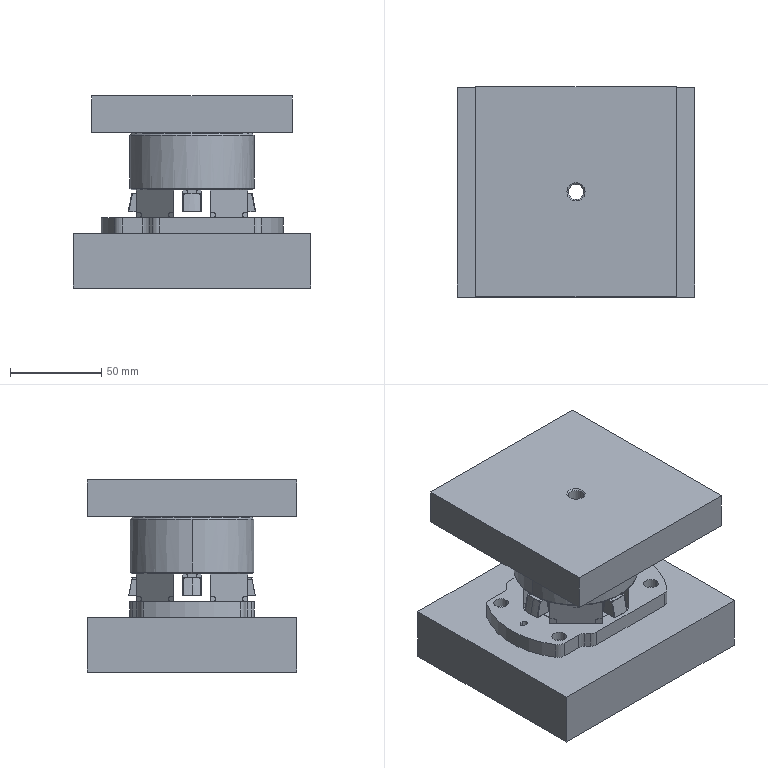NC program | NX | posted with a generic post | part box 130 x 115 x 105.2 mm
Lines 1 to 1664 of 1812, first 1463 of 1650 lines:
N10 G17 G21 G94 G90
(ADAPTIVE_MILLING_1 , TOOL : ER25-D10-50)
N12 T04 M6
N14 G54
N16 G17 G0 G90 X65.581 Y1.184 B0. C0. S6500 M3
N18 G43 Z50. H4
N20 Z-6.85
N22 G94 G1 X65.432 Y1.173 Z-7.787 F2500.
N24 X65.282 Y1.162 Z-8.158
N26 X65.133 Y1.151 Z-8.43
N28 X64.983 Y1.139 Z-8.65
N30 X64.834 Y1.128 Z-8.834
N32 X64.684 Y1.117 Z-8.992
N34 X64.534 Y1.106 Z-9.13
N36 X64.385 Y1.095 Z-9.25
N38 X64.235 Y1.084 Z-9.355
N40 X64.086 Y1.073 Z-9.448
N42 X63.936 Y1.062 Z-9.529
N44 X63.786 Y1.05 Z-9.6
N46 X63.637 Y1.039 Z-9.66
N48 X63.487 Y1.028 Z-9.712
N50 X63.338 Y1.017 Z-9.755
N52 X63.188 Y1.006 Z-9.789
N54 X63.038 Y0.995 Z-9.816
N56 X62.889 Y0.984 Z-9.835
N58 X62.739 Y0.973 Z-9.846
N60 X62.59 Y0.962 Z-9.85
N62 X60.898 Y0.836
N64 G3 X60.073 Y0.287 R1.011
N66 X59.334 Y-2.595 R8.58
N68 X59.03 Y-9.309 R68.894
N70 G1 X58.999 Y-20.218
N72 X58.998 Y-54.643
N74 G2 X57.298 Y-58.286 R5.275
N76 X53.088 Y-60.557 R9.591
N78 X47.379 Y-61.345 R26.709
N80 X37.556 Y-61.496 R223.301
N82 G1 X31.781 Y-61.5
N84 X-52.193 Y-61.498
N86 G2 X-55.736 Y-59.84 R5.295
N88 X-58.042 Y-55.63 R9.519
N90 X-58.845 Y-49.847 R26.601
N92 X-58.996 Y-39.424 R237.991
N94 G1 X-58.998 Y-34.474
N96 X-58.996 Y54.766
N98 G2 X-57.18 Y58.434 R5.368
N100 X-52.956 Y60.612 R9.75
N102 X-47.165 Y61.358 R28.291
N104 X-34.942 Y61.498 R307.021
N106 G1 X52.124 Y61.499
N108 G2 X55.836 Y59.781 R5.281
N110 X58.074 Y55.593 R9.546
N112 X58.843 Y49.956 R26.863
N114 X58.995 Y40.058 R225.033
N116 G1 X58.998 Y34.133
N118 Y3.858
N120 G2 X58.558 Y-0.729 R47.799
N122 G3 X58.039 Y-10.664 R96.401
N124 X57.999 Y-21.268 R738.972
N126 G1 X57.997 Y-51.718
N128 G2 X55.1 Y-57.334 R7.34
N130 X50.069 Y-59.612 R12.527
N132 X43.371 Y-60.37 R36.438
N134 X31.298 Y-60.498 R355.1
N136 G1 X-49.043 Y-60.499
N138 G2 X-54.865 Y-57.555 R7.352
N140 X-57.102 Y-52.6 R12.564
N142 X-57.867 Y-45.904 R36.265
N144 X-57.997 Y-33.38 R364.74
N146 G1 X-57.999 Y51.616
N148 G2 X-55.024 Y57.413 R7.314
N150 X-49.98 Y59.639 R12.698
N152 X-43.354 Y60.371 R37.226
N154 X-30.98 Y60.497 R370.258
N156 G1 X49.115 Y60.499
N158 G2 X54.867 Y57.581 R7.301
N160 X57.105 Y52.624 R12.526
N162 X57.861 Y46.077 R35.796
N164 X57.997 Y33.404 R353.751
N166 G1 X57.998 Y6.483
N168 G2 X57.547 Y-0.617 R77.039
N170 G3 X57.02 Y-14.091 R160.217
N172 G1 X57. Y-24.118
N174 X56.999 Y-48.993
N176 G2 X53.038 Y-56.516 R8.69
N178 X47.485 Y-58.685 R15.07
N180 X40.477 Y-59.377 R44.29
N182 X26.003 Y-59.498 R479.139
N184 G1 X-46.493
N186 G2 X-54.053 Y-55.478 R8.701
N188 X-56.201 Y-49.898 R15.208
N190 X-56.891 Y-42.514 R46.719
N192 X-56.997 Y-28.415 R538.22
N194 G1 Y49.066
N196 G2 X-53.012 Y56.544 R8.655
N198 X-47.599 Y58.666 R14.978
N200 X-40.443 Y59.378 R44.055
N202 X-24.694 Y59.498 R542.707
N204 G1 X46.531
N206 G2 X54.07 Y55.474 R8.673
N208 X56.194 Y49.957 R15.187
N210 X56.88 Y42.873 R45.112
N212 X56.997 Y28.399 R498.713
N214 G1 X56.995 Y8.058
N216 G2 X56.539 Y-0.562 R114.182
N218 G3 X56.012 Y-16.781 R219.905
N220 G1 X56. Y-25.018
N222 X55.999 Y-46.618
N224 G2 X55.202 Y-51.165 R11.232
N226 X50.575 Y-55.993 R10.068
N228 X44.66 Y-57.836 R18.683
N230 X36.887 Y-58.415 R60.361
N232 X22.037 Y-58.498 R765.904
N234 G1 X-44.168 Y-58.497
N236 G2 X-48.779 Y-57.649 R11.007
N238 X-53.504 Y-53.051 R10.114
N240 X-55.339 Y-47.125 R18.765
N242 X-55.921 Y-39.051 R62.317
N244 X-55.997 Y-25.852 R759.417
N246 G1 Y46.666
N248 G2 X-55.187 Y51.209 R11.083
N250 X-50.584 Y55.995 R10.052
N252 X-44.66 Y57.837 R18.699
N254 X-36.737 Y58.418 R61.322
N256 X-21.888 Y58.498 R807.199
N258 G1 X44.165 Y58.497
N260 G2 X48.709 Y57.687 R11.085
N262 X53.496 Y53.082 R10.049
N264 X55.337 Y47.158 R18.706
N266 X55.921 Y39.085 R62.102
N268 X55.997 Y25.886 R759.211
N270 G1 X55.996 Y10.011
N272 G2 X55.519 Y-0.75 R149.74
N274 G3 X55.009 Y-18.653 R271.158
N276 G1 X55. Y-26.893
N278 X54.999 Y-44.418
N280 G2 X54.496 Y-48.722 R14.697
N282 X49.785 Y-54.561 R10.27
N284 X43.719 Y-56.688 R18.043
N286 X35.807 Y-57.386 R54.254
N288 X19.683 Y-57.498 R625.027
N290 G1 X-42.017 Y-57.496
N292 G2 X-46.46 Y-56.919 R14.012
N294 X-52.181 Y-52.078 R10.365
N296 X-54.202 Y-46.131 R18.445
N298 X-54.889 Y-38.142 R55.53
N300 X-54.997 Y-22.093 R653.276
N302 G1 X-54.996 Y44.566
N304 G2 X-54.408 Y49.007 R13.879
N306 X-49.595 Y54.678 R10.344
N308 X-43.499 Y56.728 R18.571
N310 X-35.733 Y57.388 R56.178
N312 X-19.984 Y57.497 R616.787
N314 G1 X41.99
N316 G2 X46.363 Y56.955 R14.314
N318 X52.104 Y52.222 R10.284
N320 X54.202 Y46.144 R18.234
N322 X54.892 Y38.081 R55.809
N324 X54.996 Y23.682 R592.8
N326 G1 X54.995 Y11.583
N328 G2 X54.494 Y-1.098 R190.151
N330 G3 X54.007 Y-20.675 R325.437
N332 G1 X54.001 Y-27.268
N334 X54. Y-42.318
N336 G2 X53.595 Y-46.788 R18.659
N338 X48.585 Y-53.411 R10.673
N340 X42.533 Y-55.599 R18.347
N342 X34.477 Y-56.367 R52.641
N344 X17.978 Y-56.497 R567.816
N346 G1 X-40.043 Y-56.496
N348 G2 X-44.506 Y-56.036 R17.278
N350 X-50.925 Y-51.061 R10.706
N352 X-53.114 Y-44.946 R18.475
N354 X-53.863 Y-37.039 R52.944
N356 X-53.995 Y-22.566 R481.086
N358 G1 X-53.997 Y41.984
N360 G2 X-53.67 Y46.463 R21.304
N362 X-48.641 Y53.382 R10.64
N364 X-42.534 Y55.599 R18.286
N366 X-34.403 Y56.369 R53.01
N368 X-17.83 Y56.497 R581.839
N370 G1 X40.04 Y56.496
N372 G2 X44.504 Y56.041 R17.334
N374 X50.971 Y50.992 R10.714
N376 X53.132 Y44.859 R18.66
N378 X53.869 Y36.875 R54.132
N380 X53.996 Y20.002 R595.418
N382 X53.894 Y6.859 R402.358
N384 X53.332 Y-4.268 R926.663
N386 G3 X53.003 Y-23.896 R438.267
N388 G1 X53.001 Y-28.843
N390 X53. Y-40.368
N392 G2 X52.672 Y-44.923 R23.27
N394 X47.328 Y-52.337 R11.086
N396 X41.071 Y-54.58 R19.057
N398 X32.791 Y-55.363 R54.844
N400 X18.692 Y-55.496 R477.775
N402 G1 X-37.458 Y-55.497
N404 G2 X-42.168 Y-55.219 R26.666
N406 X-49.894 Y-49.73 R11.111
N408 X-52.086 Y-43.539 R19.184
N410 X-52.858 Y-35.409 R54.524
N412 X-52.995 Y-20.935 R475.03
N414 G1 X-52.996 Y40.141
N416 G2 X-52.701 Y44.774 R25.127
N418 X-47.289 Y52.363 R11.067
N420 X-41.019 Y54.591 R19.177
N422 X-32.663 Y55.367 R55.62
N424 X-15.789 Y55.496 R596.273
N426 G1 X37.961
N428 G2 X42.661 Y55.123 R21.898
N430 X49.849 Y49.812 R11.083
N432 X52.097 Y43.483 R19.174
N434 X52.86 Y35.351 R55.164
N436 X52.995 Y20.952 R480.194
N438 X52.896 Y7.553 R432.06
N440 X52.349 Y-4.038 R856.063
N442 G3 X52.003 Y-25.32 R483.268
N444 G1 X52.001 Y-37.668
N446 G2 X51.79 Y-42.759 R37.517
N448 X46.039 Y-51.312 R11.491
N450 X39.633 Y-53.572 R19.769
N452 X31.278 Y-54.358 R56.565
N454 X16.879 Y-54.495 R478.938
N456 G1 X-35.693 Y-54.496
N458 G2 X-40.63 Y-54.229 R30.471
N460 X-48.843 Y-48.484 R11.482
N462 X-51.083 Y-42.063 R19.895
N464 X-51.856 Y-33.781 R56.857
N466 X-51.995 Y-18.858 R495.156
N468 G1 X-51.996 Y37.967
N470 G2 X-51.755 Y42.981 R33.159
N472 X-46.047 Y51.309 R11.454
N474 X-39.623 Y53.573 R19.798
N476 X-31.417 Y54.352 R55.913
N478 X-16.569 Y54.495 R477.594
N480 G1 X35.69 Y54.496
N482 G2 X40.627 Y54.231 R30.554
N484 X48.809 Y48.546 R11.454
N486 X51.073 Y42.12 R19.774
N488 X51.859 Y33.69 R56.924
N490 X51.995 Y17.191 R557.858
N492 X51.491 Y-1.059 R289.671
N494 G3 X51.006 Y-23.973 R448.609
N496 G1 X51.002 Y-30.568
N498 G2 X50.955 Y-39.392 R282.827
N500 X49.869 Y-44.727 R14.734
N502 X44.416 Y-50.497 R12.086
N504 X37.952 Y-52.617 R21.22
N506 X29.367 Y-53.368 R61.75
N508 X11.668 Y-53.496 R655.381
N510 G1 X-34.432 Y-53.495
N512 G2 X-39.441 Y-53.188 R29.462
N514 X-47.818 Y-47.23 R11.811
N516 X-50.05 Y-40.812 R20.383
N518 X-50.851 Y-32.308 R57.628
N520 X-50.995 Y-15.434 R560.068
N522 G1 X-50.994 Y37.066
N524 G2 X-50.666 Y42.073 R28.129
N526 X-44.841 Y50.258 R11.75
N528 X-38.352 Y52.543 R20.23
N530 X-30.148 Y53.339 R56.098
N532 X-15.225 Y53.494 R451.589
N534 G1 X33.575 Y53.496
N536 G2 X38.817 Y53.287 R40.575
N538 X47.858 Y47.165 R11.844
N540 X50.091 Y40.588 R20.769
N542 X50.862 Y32.005 R60.068
N544 X50.883 Y8.157 R539.368
N546 X50.335 Y-4.618 R978.675
N548 G3 X50.003 Y-27.869 R586.321
N550 G2 X49.952 Y-37.967 R367.829
N552 X48.864 Y-43.454 R15.561
N554 X43.213 Y-49.462 R12.315
N556 X36.455 Y-51.636 R21.944
N558 X27.718 Y-52.371 R65.052
N560 X10.394 Y-52.496 R657.552
N562 G1 X-32.843 Y-52.494
N564 G2 X-38.078 Y-52.186 R32.006
N566 X-46.759 Y-46.072 R12.077
N568 X-49.021 Y-39.58 R20.752
N570 X-49.845 Y-30.927 R58.346
N572 X-49.993 Y-15.704 R488.743
N574 G1 X-49.995 Y34.666
N576 G2 X-49.78 Y39.983 R42.111
N578 X-43.497 Y49.305 R12.124
N580 X-36.992 Y51.539 R20.941
N582 X-28.337 Y52.349 R59.206
N584 X-11.389 Y52.495 R561.78
N586 G1 X32.84 Y52.494
N588 G2 X38.075 Y52.189 R32.147
N590 X46.727 Y46.13 R12.055
N592 X48.982 Y39.784 R20.464
N594 X49.826 Y31.435 R55.234
N596 X49.789 Y5.789 R421.475
N598 G3 X49.147 Y-10.927 R870.456
N600 X49.001 Y-33.418 R987.259
N602 G2 X48.736 Y-38.957 R39.264
N604 X42.422 Y-48.213 R12.359
N606 X35.713 Y-50.528 R21.272
N608 X26.985 Y-51.345 R60.247
N610 X12.136 Y-51.494 R479.989
N612 G1 X-30.214 Y-51.495
N614 G2 X-35.982 Y-51.294 R50.187
N616 X-43.254 Y-48.064 R12.494
N618 X-47.036 Y-41.999 R15.004
N620 X-48.533 Y-34.516 R31.851
N622 X-48.961 Y-23.653 R130.924
N624 G1 X-48.994 Y-11.278
N626 Y33.547
N628 G2 X-48.725 Y39.01 R38.045
N630 X-42.42 Y48.215 R12.339
N632 X-35.859 Y50.499 R21.139
N634 X-27.282 Y51.334 R58.29
N636 X-12.059 Y51.493 R459.036
N638 G1 X30.44 Y51.495
N640 G2 X36.132 Y51.277 R46.31
N642 X45.778 Y44.807 R12.398
N644 X48.05 Y38.083 R21.569
N646 X48.856 Y29.127 R62.376
N648 X48.489 Y-1.036 R389.187
N650 G3 X48.006 Y-27.271 R569.055
N652 G2 X47.93 Y-35.594 R208.378
N654 X46.789 Y-41.148 R16.159
N656 X40.968 Y-47.349 R12.759
N658 X34.067 Y-49.588 R22.506
N660 X25.182 Y-50.358 R65.558
N662 X10.108 Y-50.494 R538.475
N664 G1 X-28.718
N666 G2 X-34.636 Y-50.296 R53.736
N668 X-41.45 Y-47.613 R13.001
N670 X-45.722 Y-41.591 R14.405
N672 X-47.42 Y-34.231 R28.871
N674 X-47.942 Y-23.823 R106.969
N676 X-47.994 Y-9.799 R869.488
N678 G1 X-47.993 Y32.041
N680 G2 X-47.742 Y37.581 R41.91
N682 X-41.192 Y47.224 R12.603
N684 X-34.394 Y49.529 R21.846
N686 X-25.439 Y50.348 R62.488
N688 X-10.59 Y50.493 R497.634
N690 G1 X28.685 Y50.494
N692 G2 X34.603 Y50.301 R55.048
N694 X41.247 Y47.773 R13.046
N696 X45.624 Y41.83 R14.168
N698 X47.381 Y34.561 R27.899
N700 X47.929 Y24.681 R97.516
N702 X47.507 Y-0.582 R383.106
N704 G3 X47.008 Y-26.823 R579.726
N706 G2 X46.914 Y-34.545 R159.561
N708 X45.666 Y-40.227 R16.07
N710 X39.768 Y-46.352 R13.
N712 X32.791 Y-48.586 R23.001
N714 X23.756 Y-49.359 R67.317
N716 X5.382 Y-49.494 R680.95
N718 G1 X-27.968 Y-49.493
N720 G2 X-33.734 Y-49.248 R45.709
N722 X-41.226 Y-45.792 R12.9
N724 X-44.991 Y-39.646 R15.605
N726 X-46.508 Y-32.09 R32.721
N728 X-46.96 Y-20.777 R133.766
N730 G1 X-46.993 Y-8.403
N732 Y30.541
N734 G2 X-46.729 Y36.38 R43.881
N736 X-39.99 Y46.23 R12.817
N738 X-33.187 Y48.515 R22.275
N740 X-24.383 Y49.336 R62.359
N742 X-9.159 Y49.492 R480.523
N744 G1 X27.065 Y49.494
N746 G2 X33.135 Y49.32 R63.441
N748 X39.535 Y47.161 R13.717
N750 X44.401 Y41.138 R13.905
N752 X46.276 Y34.056 R26.36
N754 X46.907 Y24.332 R85.675
N756 X46.515 Y-0.353 R377.256
N758 G3 X46.006 Y-28.549 R631.975
N760 G2 X45.79 Y-34.692 R56.771
N762 X43.231 Y-41.49 R13.598
N764 X37.147 Y-46.03 R14.491
N766 X29.962 Y-47.82 R27.89
N768 X19.709 Y-48.423 R95.321
N770 X4.035 Y-48.494 R882.083
N772 G1 X-26.468 Y-48.493
N774 G2 X-32.533 Y-48.24 R48.403
N776 X-39.78 Y-45.079 R13.198
N778 X-43.839 Y-38.862 R15.32
N780 X-45.453 Y-31.327 R31.366
N782 X-45.941 Y-20.992 R116.159
N784 X-45.993 Y-6.968 R871.206
N786 G1 X-45.992 Y29.041
N788 G2 X-45.741 Y35.031 R47.705
N790 X-42.624 Y42.229 R13.188
N792 X-36.452 Y46.306 R15.221
N794 X-28.848 Y47.951 R31.174
N796 X-18.438 Y48.442 R115.943
N798 X-4.413 Y48.493 R874.688
N800 G1 X26.39
N802 G2 X32.307 Y48.269 R51.784
N804 X39.091 Y45.649 R13.47
N806 X43.529 Y39.648 R14.525
N808 X45.318 Y32.463 R27.922
N810 X45.907 Y22.886 R90.578
N812 X45.578 Y1.292 R351.9
N814 G3 X45.002 Y-28.777 R674.536
N816 G2 X44.649 Y-34.46 R37.09
N818 X37.858 Y-44.117 R13.12
N820 X30.854 Y-46.488 R22.63
N822 X21.826 Y-47.332 R63.658
N824 X6.603 Y-47.492 R480.407
N826 G1 X-24.143 Y-47.493
N828 G2 X-30.737 Y-47.304 R68.277
N830 X-37.1 Y-45.246 R14.36
N832 X-42.202 Y-39.211 R14.018
N834 X-44.209 Y-32.005 R25.961
N836 X-44.893 Y-22.21 R82.504
N838 X-44.992 Y-5.561 R847.786
N840 G1 Y27.541
N842 G2 X-44.763 Y33.608 R53.662
N844 X-42.282 Y40.279 R13.792
N846 X-36.201 Y44.933 R14.481
N848 X-28.956 Y46.787 R27.67
N850 X-18.855 Y47.413 R92.038
N852 X-3.031 Y47.492 R862.571
N854 G1 X24.919
N856 G2 X31.062 Y47.268 R55.148
N858 X37.689 Y44.846 R13.83
N860 X42.341 Y38.907 R14.343
N862 X44.245 Y31.751 R26.882
N864 X44.889 Y22.254 R83.356
N866 X44.582 Y1.484 R338.217
N868 G3 X44.002 Y-27.806 R691.633
N870 G2 X43.585 Y-33.634 R34.572
N872 X36.746 Y-43.102 R13.255
N874 X29.816 Y-45.456 R22.808
N876 X20.64 Y-46.327 R63.612
N878 X4.592 Y-46.492 R497.799
N880 G1 X-22.683 Y-46.493
N882 G2 X-29.354 Y-46.319 R75.772
N884 X-35.497 Y-44.525 R15.032
N886 X-40.956 Y-38.572 R13.792
N888 X-43.123 Y-31.34 R24.913
N890 X-43.872 Y-21.701 R75.912
N892 X-43.992 Y-4.152 R748.319
N894 G1 X-43.991 Y26.048
N896 G2 X-43.768 Y32.341 R57.737
N898 X-41.359 Y39.045 R14.141
N900 X-35.366 Y43.789 R14.449
N902 X-28.144 Y45.728 R26.971
N904 X-18.197 Y46.398 R86.187
N906 X-1.547 Y46.492 R859.438
N908 G1 X23.478
N910 G2 X29.845 Y46.267 R58.285
N912 X36.423 Y43.943 R14.17
N914 X41.291 Y37.862 R14.38
N916 X43.217 Y30.715 R26.902
N918 X43.884 Y20.918 R82.473
N920 X43.587 Y1.723 R331.857
N922 G3 X42.998 Y-27.135 R750.645
N924 G2 X42.517 Y-32.807 R31.
N926 X35.72 Y-42.044 R13.362
N928 X28.799 Y-44.423 R22.776
N930 X19.926 Y-45.305 R61.577
N932 X3.428 Y-45.491 R459.998
N934 G1 X-21.222 Y-45.492
N936 G2 X-28.192 Y-45.314 R79.378
N938 X-34.35 Y-43.535 R15.301
N940 X-39.908 Y-37.527 R13.863
N942 X-42.097 Y-30.299 R24.905
N944 X-42.853 Y-21.037 R73.224
N946 X-42.991 Y-2.663 R685.472
N948 G1 Y24.612
N950 G2 X-42.768 Y31.13 R61.328
N952 X-40.536 Y37.668 R14.509
N954 X-34.546 Y42.643 R14.311
N956 X-27.345 Y44.668 R26.291
N958 X-17.702 Y45.378 R80.287
N960 X-0.153 Y45.491 R787.546
N962 G1 X22.022
N964 G2 X28.541 Y45.277 R63.393
N966 X35.029 Y43.126 R14.609
N968 X40.142 Y37.045 R14.278
N970 X42.179 Y29.769 R26.396
N972 X42.866 Y20.049 R78.87
N974 X42.59 Y1.904 R320.779
N976 G3 X42.002 Y-25.94 R764.476
N978 G2 X41.495 Y-31.759 R31.273
N980 X34.543 Y-41.077 R13.499
N982 X27.532 Y-43.44 R23.299
N984 X18.581 Y-44.309 R63.53
N986 X2.083 Y-44.491 R472.545
N988 G1 X-20.617 Y-44.492
N990 G2 X-27.286 Y-44.284 R67.55
N992 X-33.607 Y-42.318 R15.082
N994 X-39.036 Y-36.14 R14.177
N996 X-41.133 Y-28.887 R25.936
N998 X-41.858 Y-19.622 R76.628
N1000 X-41.991 Y-1.248 R716.06
N1002 G1 Y23.252
N1004 G2 X-41.769 Y29.92 R64.273
N1006 X-39.67 Y36.351 R14.856
N1008 X-33.564 Y41.572 R14.328
N1010 X-26.378 Y43.634 R26.093
N1012 X-16.962 Y44.363 R77.563
N1014 X0.587 Y44.491 R702.6
N1016 G1 X20.737
N1018 G2 X27.331 Y44.28 R66.319
N1020 X33.712 Y42.256 R15.014
N1022 X39.007 Y36.197 R14.205
N1024 X41.133 Y28.877 R25.835
N1026 X41.845 Y19.235 R75.068
N1028 X41.586 Y1.914 R312.099
N1030 G3 X41.005 Y-24.896 R815.631
N1032 G2 X40.476 Y-30.713 R30.956
N1034 X33.582 Y-39.993 R13.573
N1036 X26.438 Y-42.427 R23.315
N1038 X17.188 Y-43.314 R64.771
N1040 X1.515 Y-43.49 R466.288
N1042 G1 X-18.56 Y-43.491
N1044 G2 X-25.681 Y-43.324 R88.501
N1046 X-31.87 Y-41.669 R16.168
N1048 X-37.787 Y-35.522 R13.952
N1050 X-40.036 Y-28.311 R24.748
N1052 X-40.844 Y-18.827 R71.763
N1054 X-40.99 Y-0.378 R660.624
N1056 G1 Y21.947
N1058 G2 X-40.766 Y28.765 R66.632
N1060 X-38.652 Y35.272 R15.041
N1062 X-32.389 Y40.598 R14.43
N1064 X-25.04 Y42.659 R26.721
N1066 X-15.397 Y43.371 R81.452
N1068 X2.152 Y43.49 R760.455
N1070 G1 X19.377
N1072 G2 X26.121 Y43.282 R69.642
N1074 X32.39 Y41.384 R15.393
N1076 X37.974 Y35.149 R14.213
N1078 X40.123 Y27.759 R25.989
N1080 X40.835 Y17.742 R75.687
N1082 X40.587 Y2.07 R313.823
N1084 G3 X40.003 Y-24.076 R936.375
N1086 G2 X39.394 Y-29.959 R28.901
N1088 X32.488 Y-38.99 R13.675
N1090 X25.264 Y-41.431 R23.626
N1092 X15.789 Y-42.321 R66.565
N1094 X-0.259 Y-42.489 R499.202
N1096 G1 X-17.184 Y-42.491
N1098 G2 X-24.455 Y-42.329 R94.652
N1100 X-30.596 Y-40.757 R16.613
N1102 X-36.756 Y-34.479 R13.991
N1104 X-39.04 Y-27.129 R25.02
N1106 X-39.835 Y-17.87 R71.829
N1108 X-39.988 Y-2.196 R528.715
N1110 G1 X-39.99 Y19.679
N1112 G2 X-39.828 Y26.95 R94.691
N1114 X-38.261 Y33.089 R16.655
N1116 X-32.049 Y39.218 R13.964
N1118 X-24.842 Y41.503 R24.633
N1120 X-15.361 Y42.335 R70.552
N1122 X0.313 Y42.489 R529.364
N1124 G1 X17.163 Y42.49
N1126 G2 X24.509 Y42.324 R93.19
N1128 X30.574 Y40.767 R16.597
N1130 X36.685 Y34.614 R13.929
N1132 X39. Y27.338 R24.471
N1134 X39.8 Y17.404 R68.239
N1136 X39.586 Y2.182 R292.402
N1138 G3 X39.016 Y-22.732 R924.824
N1140 G2 X38.431 Y-28.694 R30.76
N1142 X31.527 Y-37.915 R13.755
N1144 X24.321 Y-40.394 R23.438
N1146 X15.149 Y-41.299 R64.035
N1148 X-1.724 Y-41.489 R474.742
N1150 G1 X-16.624 Y-41.49
N1152 G2 X-23.669 Y-41.295 R79.458
N1154 X-30.04 Y-39.474 R16.076
N1156 X-35.892 Y-33.113 R14.313
N1158 X-38.07 Y-25.806 R25.938
N1160 X-38.836 Y-16.619 R74.137
N1162 X-38.989 Y1.754 R640.868
N1164 G1 Y19.129
N1166 G2 X-38.794 Y26.174 R79.205
N1168 X-37.043 Y32.413 R16.151
N1170 X-30.728 Y38.333 R14.227
N1172 X-23.283 Y40.572 R25.858
N1174 X-14.096 Y41.337 R74.296
N1176 X4.278 Y41.49 R642.255
N1178 G1 X16.703
N1180 G2 X23.822 Y41.279 R75.338
N1182 X30.175 Y39.398 R15.833
N1184 X35.863 Y33.168 R14.292
N1186 X38.064 Y25.789 R25.683
N1188 X38.787 Y15.773 R71.98
N1190 X38.559 Y1.451 R314.085
N1192 G3 X38.026 Y-21.614 R937.928
N1194 G2 X37.47 Y-27.429 R31.95
N1196 X30.367 Y-36.956 R13.89
N1198 X23.146 Y-39.403 R23.817
N1200 X13.823 Y-40.304 R65.591
N1202 X-3.05 Y-40.489 R490.322
N1204 G1 X-15.4 Y-40.49
N1206 G2 X-22.52 Y-40.295 R81.489
N1208 X-28.772 Y-38.573 R16.439
N1210 X-34.784 Y-32.236 R14.26
N1212 X-37.024 Y-24.946 R25.507
N1214 X-37.832 Y-15.537 R72.699
N1216 X-37.987 Y0.137 R530.923
N1218 G1 X-37.989 Y17.062
N1220 G2 X-37.822 Y24.708 R100.438
N1222 X-36.25 Y30.923 R17.086
N1224 X-30.04 Y37.126 R14.087
N1226 X-22.783 Y39.465 R24.694
N1228 X-13.379 Y40.32 R69.178
N1230 X2.594 Y40.488 R504.568
N1232 G1 X15.394 Y40.489
N1234 G2 X22.439 Y40.302 R83.286
N1236 X28.631 Y38.646 R16.646
N1238 X34.669 Y32.459 R14.148
N1240 X36.984 Y25.112 R24.859
N1242 X37.746 Y15.551 R66.332
N1244 X37.557 Y1.528 R285.626
N1246 G3 X37.037 Y-20.495 R955.405
N1248 G2 X36.463 Y-26.383 R32.033
N1250 X29.333 Y-35.932 R13.973
N1252 X22.105 Y-38.388 R23.981
N1254 X12.932 Y-39.293 R64.722
N1256 X-3.566 Y-39.488 R452.973
N1258 X-18.84 Y-39.442 R815.559
N1260 X-24.709 Y-38.726 R25.812
N1262 X-33.352 Y-31.959 R13.845
N1264 X-35.855 Y-24.761 R23.505
N1266 X-36.785 Y-15.592 R63.146
N1268 X-36.986 Y0.906 R442.685
N1270 G1 X-36.989 Y15.806
N1272 G2 X-36.837 Y23.378 R108.462
N1274 X-35.419 Y29.482 R17.849
N1276 X-29.08 Y36.061 R14.083
N1278 X-21.687 Y38.461 R24.757
N1280 X-12.283 Y39.317 R69.669
N1282 X3.39 Y39.487 R490.541
N1284 X18.74 Y39.445 R846.733
N1286 X24.684 Y38.733 R26.201
N1288 X33.41 Y31.852 R13.854
N1290 X35.878 Y24.549 R23.734
N1292 X36.705 Y15.145 R61.2
N1294 X36.526 Y0.672 R277.373
N1296 G3 X36.048 Y-19.452 R995.014
N1298 G2 X35.426 Y-25.485 R31.538
N1300 X28.242 Y-34.942 R14.055
N1302 X20.944 Y-37.397 R24.256
N1304 X11.396 Y-38.308 R67.239
N1306 X-4.652 Y-38.487 R481.392
N1308 X-17.752 Y-38.44 R626.042
N1310 X-23.765 Y-37.685 R25.707
N1312 X-32.364 Y-30.862 R13.934
N1314 X-34.869 Y-23.575 R23.875
N1316 X-35.801 Y-14.029 R65.971
N1318 X-35.986 Y2.469 R478.658
N1320 G1 X-35.988 Y15.344
N1322 G2 X-35.793 Y22.764 R86.66
N1324 X-34.117 Y29.027 R16.842
N1326 X-27.861 Y35.137 R14.303
N1328 X-20.377 Y37.495 R25.368
N1330 X-10.67 Y38.332 R73.36
N1332 X5.003 Y38.487 R541.434
N1334 X17.878 Y38.435 R561.687
N1336 X23.814 Y37.672 R25.169
N1338 X32.349 Y30.883 R13.913
N1340 X34.841 Y23.597 R23.544
N1342 X35.679 Y14.044 R60.582
N1344 X35.523 Y0.696 R271.517
N1346 G3 X35.076 Y-17.883 R922.118
N1348 G2 X34.52 Y-24. R35.78
N1350 X27.232 Y-33.91 R14.157
N1352 X19.798 Y-36.405 R24.413
N1354 X10.174 Y-37.31 R68.43
N1356 X-5.799 Y-37.487 R487.3
N1358 X-17.198 Y-37.418 R369.817
N1360 X-23.12 Y-36.558 R23.511
N1362 X-31.377 Y-29.767 R14.015
N1364 X-33.88 Y-22.414 R24.141
N1366 X-34.786 Y-13.241 R65.321
N1368 X-34.985 Y3.257 R450.921
N1370 X-34.947 Y18.832 R901.281
N1372 X-34.286 Y24.784 R28.078
N1374 X-27.243 Y33.892 R14.03
N1376 X-19.881 Y36.386 R24.204
N1378 X-10.708 Y37.287 R65.689
N1380 X5.115 Y37.484 R436.649
N1382 X16.89 Y37.43 R454.079
N1384 X22.895 Y36.624 R24.798
N1386 X31.367 Y29.78 R13.989
N1388 X33.845 Y22.418 R23.761
N1390 X34.655 Y12.712 R61.966
N1392 X34.485 Y-0.486 R292.826
N1394 G3 X34.093 Y-16.764 R926.138
N1396 G2 X33.537 Y-22.881 R36.414
N1398 X26.134 Y-32.931 R14.256
N1400 X18.835 Y-35.381 R24.513
N1402 X9.362 Y-36.297 R67.056
N1404 X-5.486 Y-36.484 R435.045
N1406 X-15.985 Y-36.421 R340.94
N1408 X-21.984 Y-35.575 R24.164
N1410 X-30.293 Y-28.854 R14.058
N1412 X-32.798 Y-21.74 R23.604
N1414 X-33.772 Y-12.425 R62.519
N1416 X-33.982 Y2.423 R385.252
N1418 X-33.944 Y17.772 R883.831
N1420 X-33.263 Y23.797 R27.895
N1422 X-26.222 Y32.867 R14.095
N1424 X-18.94 Y35.356 R24.137
N1426 X-9.394 Y36.294 R66.165
N1428 X6.504 Y36.482 R460.788
N1430 X16.558 Y36.395 R239.895
N1432 X22.601 Y35.376 R21.634
N1434 X30.324 Y28.78 R14.016
N1436 X32.804 Y21.479 R23.61
N1438 X33.612 Y12.299 R59.237
N1440 X33.471 Y-0.824 R271.747
N1442 G3 X33.114 Y-15.57 R935.742
N1444 G2 X32.556 Y-21.762 R37.562
N1446 X25.123 Y-31.906 R14.319
N1448 X17.674 Y-34.394 R24.698
N1450 X8.05 Y-35.303 R68.545
N1452 X-14.435 Y-35.435 R553.78
N1454 X-20.524 Y-34.683 R26.504
N1456 X-29.383 Y-27.635 R14.157
N1458 X-31.843 Y-20.422 R24.211
N1460 X-32.783 Y-11.027 R65.269
N1462 X-32.983 Y4.795 R433.633
N1464 X-32.927 Y17.17 R481.898
N1466 X-32.12 Y23.251 R25.381
N1468 X-25.287 Y31.795 R14.102
N1470 X-18.094 Y34.309 R23.842
N1472 X-8.628 Y35.277 R63.633
N1474 G3 X-6.156 Y35.381 R49.75
N1476 X-5.398 Y35.716 R6.583
N1478 G2 X-2.68 Y36.23 R7.577
N1480 G1 X2.68
N1482 G2 X4.841 Y35.94 R11.012
N1484 G3 X10.069 Y35.556 R39.757
N1486 G2 X16.865 Y35.306 R115.8
N1488 X23.085 Y33.74 R17.727
N1490 X29.565 Y27.267 R14.363
N1492 X31.897 Y19.774 R24.971
N1494 X32.604 Y9.834 R67.287
N1496 X32.351 Y-5.243 R448.479
N1498 X32.048 Y-16.53 R586.308
N1500 X31.081 Y-22.586 R24.188
N1502 X24.171 Y-30.851 R14.302
N1504 X16.875 Y-33.341 R24.406
N1506 X7.329 Y-34.283 R64.944
N1508 G3 X6.137 Y-34.375 R5.284
N1510 G2 X3.661 Y-35.165 R8.381
N1512 G1 X2.68 Y-35.23
N1514 X-2.681
N1516 X-3.89 Y-35.131
N1518 G3 X-7.299 Y-34.667 R16.642
N1520 X-14.193 Y-34.418 R501.263
N1522 G2 X-20.176 Y-33.474 R23.326
N1524 X-28.278 Y-26.767 R14.178
N1526 X-30.826 Y-19.425 R24.06
N1528 X-31.782 Y-9.882 R65.051
N1530 X-31.982 Y6.972 R469.979
N1532 X-31.892 Y16.888 R230.689
N1534 X-30.885 Y22.935 R22.089
N1536 X-24.25 Y30.785 R14.174
N1538 X-16.984 Y33.314 R24.002
N1540 X-8.532 Y34.235 R62.306
N1542 G3 X-7.532 Y34.441 R2.192
N1544 G2 X-5.957 Y35.45 R7.608
N1546 G3 X-7.626 Y34.357 R7.411
N1548 G2 X-9.716 Y33.778 R7.145
N1550 G3 X-15.564 Y32.918 R409.187
N1552 X-22.649 Y30.761 R26.48
N1554 X-29.235 Y24.526 R14.347
N1556 X-31.046 Y18.141 R18.177
N1558 X-31.372 Y10.352 R73.598
N1560 G1 X-31.375 Y3.542
N1562 X-31.551 Y1.763
N1564 X-31.586 Y-0.93
N1566 G2 X-31.222 Y-8.676 R146.448
N1568 G3 X-30.394 Y-18.083 R74.704
N1570 X-28.186 Y-25.302 R25.638
N1572 X-18.481 Y-33.055 R14.248
N1574 X-12.389 Y-33.824 R32.737
N1576 G2 X-6.618 Y-34.165 R114.081
N1578 X-6.169 Y-34.362 R1.593
N1580 G1 X-5.066 Y-34.837
N1582 X-4.411 Y-35.001
N1584 G2 X-6.756 Y-34.003 R6.935
N1586 G3 X-9.69 Y-33.238 R10.532
N1588 G2 X-15.112 Y-32.572 R789.84
N1590 X-21.168 Y-30.671 R18.113
N1592 X-27.289 Y-24.01 R14.63
N1594 X-29.452 Y-16.618 R26.691
N1596 X-30.145 Y-9.454 R72.861
N1598 X-30.97 Y-6.277 R46.807
N1600 G1 X-31.392 Y-3.617
N1602 X-31.425 Y-3.168
N1604 X-31.392 Y-3.617
N1606 X-30.97 Y-6.277
N1608 X-30.323 Y-8.892
N1610 G2 X-29.428 Y-12.656 R16.222
N1612 G3 X-28.247 Y-19.207 R61.389
N1614 X-25.346 Y-25.768 R19.763
N1616 X-17.733 Y-31.156 R14.283
N1618 X-12.225 Y-32.269 R34.909
N1620 G2 X-8.024 Y-33.071 R27.715
N1622 G1 X-7.711 Y-33.243
N1624 G3 X-6.613 Y-34.079 R4.624
N1626 G2 X-7.711 Y-33.243 R4.624
N1628 G3 X-9.66 Y-32.146 R4.873
N1630 X-13.881 Y-31.07 R42.981
N1632 G2 X-19.459 Y-29.109 R21.687
N1634 X-25.711 Y-22.383 R14.759
N1636 X-27.798 Y-15.746 R27.533
N1638 G3 X-28.086 Y-14.439 R9.07
N1640 G1 X-28.374 Y-13.909
N1642 X-29.456 Y-11.442
N1644 X-29.963 Y-9.951
N1646 X-29.456 Y-11.442
N1648 X-28.374 Y-13.909
N1650 G2 X-27.074 Y-16.927 R13.526
N1652 G3 X-25.028 Y-22.115 R33.239
N1654 X-16.713 Y-29.423 R15.05
N1656 X-11.73 Y-30.93 R54.82
N1658 G2 X-8.868 Y-32.002 R13.648
N1660 X-8.077 Y-32.916 R5.783
N1662 G1 X-8.021 Y-32.966
N1664 G3 X-9.111 Y-31.676 R24.174
N1666 X-11.552 Y-30.295 R8.55
N1668 G2 X-15.903 Y-28.599 R183.425
N1670 X-24.256 Y-20.699 R16.139
N1672 G1 X-24.866 Y-19.454
N1674 X-25.602 Y-18.523
N1676 X-27.087 Y-16.275
N1678 X-27.875 Y-14.826
N1680 X-27.087 Y-16.275
N1682 X-25.602 Y-18.523
N1684 G2 X-22.254 Y-22.81 R757.019
N1686 G3 X-15.386 Y-27.993 R18.601
N1688 G2 X-11.238 Y-29.822 R350.011
N1690 X-9.47 Y-30.917 R8.127
N1692 X-8.832 Y-31.982 R9.455
N1694 G3 X-9.719 Y-30.48 R15.173
N1696 X-10.532 Y-29.783 R2.282
N1698 G2 X-13.256 Y-28.685 R51.756
N1700 G1 X-15.65 Y-27.452
N1702 X-17.932 Y-26.02
N1704 X-20.082 Y-24.398
N1706 X-22.087 Y-22.599
N1708 X-23.932 Y-20.636
N1710 X-22.087 Y-22.599
N1712 X-20.082 Y-24.398
N1714 X-17.932 Y-26.02
N1716 X-15.65 Y-27.452
N1718 X-13.256 Y-28.685
N1720 G3 X-10.532 Y-29.783 R51.756
N1722 G2 X-9.531 Y-30.701 R1.332
N1724 G1 X-9.441 Y-30.907
N1726 G3 X-9.889 Y-30.09 R2.315
N1728 X-10.437 Y-29.812 R1.389
N1730 G2 X-9.889 Y-30.09 R1.316
N1732 X-9.623 Y-30.475 R1.232
N1734 G3 X-8.077 Y-32.916 R8.267
N1736 X-6.169 Y-34.362 R8.671
N1738 X-3.89 Y-35.131 R8.659
N1740 G1 X-2.681 Y-35.23
N1742 X2.68
N1744 G3 X6.006 Y-34.43 R7.633
N1746 G2 X7.481 Y-33.974 R4.309
N1748 X12.928 Y-33.295 R106.683
N1750 G3 X20.398 Y-31.707 R36.098
N1752 X26.9 Y-27.8 R16.859
N1754 X30.764 Y-20.487 R14.68
N1756 X31.5 Y-13.937 R37.525
N1758 X32. Y7.467 R922.126
N1760 X31.515 Y17.798 R83.917
N1762 X29.633 Y25.342 R28.228
N1764 X24.642 Y31.777 R14.876
N1766 X18.066 Y34.36 R15.701
N1768 X12.017 Y34.877 R47.153
N1770 G2 X6.542 Y35.194 R71.485
N1772 X5.4 Y35.716 R10.605
N1774 G1 X4.517 Y36.
N1776 G2 X6.75 Y35.016 R7.702
N1778 G3 X9.726 Y34.252 R10.508
N1780 X15.121 Y33.69 R295.859
N1782 G2 X21.14 Y32.195 R20.625
N1784 X28.099 Y25.384 R14.198
N1786 X30.31 Y18.006 R24.94
N1788 X30.956 Y8.436 R67.601
N1790 G1 X30.973 Y6.154
N1792 X31.138 Y5.381
N1794 G2 X31.598 Y0.323 R37.009
N1796 X31.242 Y-4.744 R37.009
N1798 G3 X30.768 Y-8.774 R25.821
N1800 G2 X30.306 Y-16.204 R202.362
N1802 X28.858 Y-22.388 R21.064
N1804 X22.075 Y-29.526 R14.368
N1806 X14.81 Y-31.862 R25.826
N1808 X8.964 Y-32.764 R369.935
N1810 G3 X7.975 Y-33.034 R2.878
N1812 G1 X6.958 Y-33.879
N1814 X6.114 Y-34.368
N1816 X6.958 Y-33.879
N1818 G2 X8.172 Y-32.884 R13.538
N1820 X10.689 Y-32.067 R9.747
N1822 G3 X16.313 Y-30.886 R158.252
N1824 X22.799 Y-28.202 R21.46
N1826 X28.806 Y-19.954 R14.327
N1828 X29.841 Y-13.599 R31.65
N1830 G1 X30.134 Y-9.486
N1832 X30.759 Y-7.24
N1834 X31.058 Y-5.694
N1836 X30.759 Y-7.24
N1838 G2 X29.525 Y-11.35 R59.714
N1840 G3 X28.644 Y-15.816 R60.402
N1842 G2 X26.839 Y-21.597 R21.477
N1844 X20.045 Y-28.166 R14.724
N1846 X14.099 Y-30.217 R28.579
N1848 G3 X9.823 Y-31.343 R51.493
N1850 X8.916 Y-31.845 R1.895
N1852 G2 X7.947 Y-33.048 R11.997
N1854 G3 X8.858 Y-31.921 R10.172
N1856 G2 X9.602 Y-31.251 R1.692
N1858 X12.754 Y-30.041 R15.247
N1860 G3 X18.102 Y-28.266 R49.659
N1862 X24.266 Y-23.901 R16.034
N1864 X27.411 Y-17.752 R16.49
N1866 X28.312 Y-14.03 R68.985
N1868 X29.71 Y-10.759 R42.866
N1870 G2 X28.077 Y-14.5 R39.869
N1872 G3 X26.627 Y-17.479 R21.825
N1874 G2 X23.692 Y-22.533 R20.262
N1876 X16.701 Y-27.459 R18.303
N1878 X11.946 Y-29.237 R151.915
N1880 G3 X9.841 Y-30.267 R10.764
N1882 X9.427 Y-30.939 R1.644
N1884 G1 X8.901 Y-31.848
N1886 G3 X9.621 Y-30.479 R8.432
N1888 G2 X10.763 Y-29.71 R1.501
N1890 G3 X15.976 Y-27.274 R35.897
N1892 X20.885 Y-24.181 R27.195
N1894 X24.574 Y-19.829 R16.767
N1896 X27.562 Y-15.408 R28.424
N1898 G2 X24.574 Y-19.829 R28.424
N1900 G1 X23.941 Y-20.625
N1902 G2 X21.133 Y-23.494 R40.052
N1904 X17.117 Y-26.562 R36.995
N1906 X12.885 Y-28.854 R37.452
N1908 G1 X10.763 Y-29.71
N1910 G3 X9.841 Y-30.122 R1.754
N1912 X9.601 Y-30.529 R1.788
N1914 X10.089 Y-31.801 R1.
N1916 X10.667 Y-31.898 Z-9.82 R1.102
N1918 G1 X12.037 Y-31.841 Z-9.75
N1920 X13.455 Y-31.783 F15000.
N1922 G3 X13.871 Y-31.673 R1.048
N1924 G1 X15.325 Y-30.927
N1926 X16.774 Y-30.17
N1928 G3 X20.723 Y-27.633 R34.131
N1930 X25.273 Y-23.563 R29.439
N1932 X27.095 Y-21.492 R46.775
N1934 X29.955 Y-17.166 R28.374
N1936 X32.813 Y-10.807 R42.022
N1938 X33.671 Y-7.805 R31.062
N1940 X34.357 Y-4.378 R45.009
N1942 X34.624 Y-1.45 R25.49
N1944 G1 X34.801 Y3.943
N1946 G3 X33.988 Y4.959 R1.
N1948 G1 X33.681 Y5.017
N1950 X31.75 Y5.384 Z-9.85 F2500.
N1952 G2 X30.973 Y6.154 R1.001
N1954 X30.395 Y10.397 R23.128
N1956 G3 X29.628 Y18.068 R74.126
N1958 X27.366 Y25.114 R23.364
N1960 X18.646 Y32.183 R14.148
N1962 X12.902 Y33.254 R34.126
N1964 G2 X8.329 Y34.001 R33.838
N1966 X7.568 Y34.402 R1.369
N1968 G3 X6.568 Y35.119 R8.941
N1970 G2 X7.992 Y33.988 R7.366
N1972 G3 X10.497 Y32.929 R7.427
N1974 X15.305 Y31.908 R127.121
N1976 G2 X21.109 Y29.729 R18.705
N1978 X26.78 Y23.167 R14.633
N1980 X28.779 Y15.887 R26.574
N1982 X29.239 Y11.939 R217.149
N1984 G1 X29.868 Y10.318
N1986 X30.605 Y7.867
N1988 X30.731 Y7.28
N1990 G3 X29.256 Y11.883 R28.606
N1992 G2 X28.397 Y15.042 R15.846
N1994 G3 X26.926 Y20.857 R40.48
N1996 X22.875 Y27.281 R15.953
N1998 X16.746 Y30.719 R15.885
N2000 X11.644 Y32.045 R88.404
N2002 G2 X8.821 Y33.061 R11.888
N2004 X8.459 Y33.482 R1.743
N2006 G1 X7.833 Y34.129
N2008 G2 X8.773 Y33.02 R5.391
N2010 G3 X10.718 Y31.734 R5.389
N2012 X14.932 Y30.253 R51.778
N2014 G2 X20.37 Y27.591 R19.588
N2016 X25.429 Y21.033 R15.536
N2018 X26.914 Y16.543 R32.642
N2020 G1 X27.812 Y15.002
N2022 G2 X29.044 Y12.423 R48.268
N2024 G3 X26.614 Y17.023 R33.11
N2026 G2 X24.987 Y20.504 R106.075
N2028 G3 X20.522 Y26.391 R16.794
N2030 X15.093 Y29.413 R19.955
N2032 G2 X10.911 Y31.082 R67.169
N2034 X9.416 Y32.006 R5.673
N2036 X9.178 Y32.424 R2.257
N2038 G1 X8.756 Y33.044
N2040 G2 X9.403 Y31.927 R4.26
N2042 G3 X11.091 Y30.416 R5.012
N2044 X14.973 Y28.442 R47.221
N2046 G2 X20.351 Y24.796 R19.757
N2048 X22.639 Y22.01 R18.642
N2050 G1 X23.383 Y21.256
N2052 X25.026 Y19.293
N2054 G2 X26.621 Y17.011 R86.798
N2056 G3 X25.026 Y19.293 R86.798
N2058 G1 X23.383 Y21.256
N2060 X21.585 Y23.079
N2062 X19.646 Y24.75
N2064 X17.578 Y26.259
N2066 X15.395 Y27.596
N2068 G2 X11.453 Y29.635 R80.178
N2070 X9.868 Y30.873 R6.069
N2072 X9.397 Y31.941 R34.872
N2074 X9.808 Y30.85 R4.287
N2076 G3 X10.725 Y29.724 R2.207
N2078 G1 X13.111 Y28.752
N2080 X10.583 Y29.772
N2082 G2 X9.8 Y30.883 R1.391
N2084 G3 X10.219 Y29.981 R1.594
N2086 X10.658 Y29.746 R1.551
N2088 X11.9 Y30.32 R1.
N2090 X11.969 Y30.913 Z-9.819 R1.379
N2092 G1 X11.937 Y32.275 Z-9.75
N2094 X11.907 Y33.592 F15000.
N2096 G3 X11.802 Y34.016 R1.044
N2098 G1 X11.411 Y34.778
N2100 G3 X10.801 Y35.53 R3.393
N2102 G1 X9.975 Y36.292
N2104 X9.139 Y37.044
N2106 G3 X6.542 Y38.537 R9.054
N2108 X4.176 Y39.143 R11.669
N2110 G1 X3.447 Y39.237
N2112 X2.714 Y39.298
N2114 X-0.805 Y39.493
N2116 G3 X-4.568 Y39.136 R12.656
N2118 G1 X-6.423 Y38.673
N2120 G3 X-7.18 Y37.742 R1.
N2122 G1 X-7.185 Y37.604
N2124 X-7.263 Y35.64 Z-9.85 F2500.
N2126 X-7.275 Y35.277
N2128 X-7.303 Y34.914
N2130 G2 X-7.567 Y34.403 R1.011
N2132 X-8.902 Y33.673 R3.352
N2134 X-12.524 Y32.844 R25.096
N2136 G3 X-18.805 Y31.482 R51.608
N2138 X-25.104 Y28.24 R17.839
N2140 X-29.712 Y20.861 R14.317
N2142 X-30.638 Y14.264 R30.67
N2144 X-30.782 Y7.135 R209.26
N2146 G1 X-31.286 Y4.444
N2148 X-31.382 Y3.473
N2150 X-31.286 Y4.444
N2152 X-30.782 Y7.135
N2154 G3 X-29.864 Y12.092 R20.827
N2156 G2 X-29.173 Y18.033 R63.336
N2158 X-26.665 Y24.41 R16.389
N2160 X-20.364 Y29.487 R14.97
N2162 X-14.353 Y31.37 R30.835
N2164 G3 X-9.79 Y32.488 R50.255
N2166 X-8.855 Y32.934 R2.463
N2168 G1 X-8.457 Y33.484
N2170 X-7.622 Y34.346
N2172 X-8.457 Y33.484
N2174 G2 X-9.041 Y32.721 R3.204
N2176 X-11.439 Y31.614 R7.969
N2178 X-16.408 Y30.215 R700.509
N2180 G3 X-22.387 Y27.468 R20.975
N2182 X-27.95 Y19.615 R14.416
N2184 X-29.028 Y13.949 R32.611
N2186 G2 X-29.308 Y11.791 R22.856
N2188 G3 X-30.317 Y8.821 R24.237
N2190 G2 X-28.734 Y13.15 R28.393
N2192 G3 X-27.645 Y16.905 R46.327
N2194 G2 X-25.364 Y22.348 R19.624
N2196 X-19.079 Y27.796 R15.297
N2198 X-14.031 Y29.728 R36.184
N2200 G3 X-10.238 Y31.152 R25.737
N2202 X-9.467 Y31.786 R1.592
N2204 G2 X-8.797 Y32.984 R4.28
N2206 G3 X-9.563 Y31.582 R5.982
N2208 G2 X-11.108 Y30.419 R4.508
N2210 X-14.874 Y28.864 R36.403
N2212 G3 X-20.348 Y26.218 R26.516
N2214 X-26.116 Y19. R15.355
N2216 X-27.153 Y16.121 R69.81
N2218 G1 X-27.646 Y15.306
N2220 X-28.734 Y13.15
N2222 G2 X-25.56 Y18.571 R34.503
N2224 X-22.251 Y22.945 R24.275
N2226 X-16.892 Y26.69 R19.931
N2228 X-11.398 Y29.468 R31.611
N2230 G3 X-10.066 Y30.324 R5.381
N2232 X-9.705 Y31.26 R2.184
N2234 G1 X-9.519 Y31.67
N2236 G3 X-9.907 Y30.495 R4.915
N2238 G2 X-10.856 Y29.677 R1.457
N2240 G1 X-11.552 Y29.396
N2242 X-10.425 Y29.829
N2244 G3 X-9.884 Y30.57 R1.096
N2246 G2 X-10.425 Y29.829 R1.118
N2248 G3 X-18.413 Y25.681 R32.984
N2250 X-24.992 Y19.337 R32.993
N2252 G1 X-25.777 Y18.239
N2254 G2 X-27.034 Y17.915 R1.01
N2256 G1 X-28.512 Y18.62
N2258 X-28.647 Y18.684 Z-9.846
N2260 X-28.782 Y18.749 Z-9.835
N2262 X-28.918 Y18.814 Z-9.816
N2264 X-29.053 Y18.878 Z-9.789
N2266 X-29.189 Y18.943 Z-9.755
N2268 X-29.324 Y19.008 Z-9.712
N2270 X-29.459 Y19.072 Z-9.66
N2272 X-29.595 Y19.137 Z-9.6
N2274 X-29.73 Y19.201 Z-9.529
N2276 X-29.865 Y19.266 Z-9.448
N2278 X-30.001 Y19.331 Z-9.355
N2280 X-30.136 Y19.395 Z-9.25
N2282 X-30.272 Y19.46 Z-9.13
N2284 X-30.407 Y19.524 Z-8.992
N2286 X-30.542 Y19.589 Z-8.834
N2288 X-30.678 Y19.654 Z-8.65
N2290 X-30.813 Y19.718 Z-8.43
N2292 X-30.948 Y19.783 Z-8.158
N2294 X-31.084 Y19.848 Z-7.787
N2296 X-31.219 Y19.912 Z-6.85
N2298 G0 Z50.
N2300 M5
(FLOOR_FACING , TOOL : ER25-D10-50_G)
N2302 T05 M6
N2304 G54
N2306 G17 G0 G90 X63.2 Y-24.312 B0. C0. S6500 M3
N2308 G43 Z50. H5
N2310 Z-7.
N2312 G94 G1 Z-10. F800.
N2314 X55.2
N2316 G3 X52.7 Y-26.812 R2.5
N2318 G1 Y-55.2
N2320 X-52.7
N2322 Y55.2
N2324 X52.7
N2326 Y-26.812
N2328 X45.2
N2330 Y-47.7
N2332 X-45.2
N2334 Y47.7
N2336 X45.2
N2338 Y-26.812
N2340 X37.7
N2342 Y-40.2
N2344 X-37.7
N2346 Y-9.47
N2348 X-30.2
N2350 G3 X-10.757 Y-29.766 R31.65
N2352 X-9.842 Y-30.005 R5.2
N2354 X-8.341 Y-32.7 R7.5
N2356 X-3.958 Y-35.17 R7.5
N2358 G1 X-3.926 Y-35.188
N2360 X-3.958 Y-35.17
N2362 G2 X-8.341 Y-32.7 R7.5
N2364 G1 X-30.2
N2366 Y-25.423
N2368 X-25.7
N2370 G3 X-22.618 Y-28.2 R36.15
N2372 G1 X-25.7
N2374 Y-25.423
N2376 X-30.2
N2378 Y-9.47
N2380 G2 X-31.315 Y-4.596 R31.65
N2382 X-31.315 Y4.596 R31.65
N2384 X-32.7 Y5.14 R5.
N2386 G1 Y-5.14
N2388 G2 X-31.315 Y-4.596 R5.
N2390 G3 X-30.2 Y-9.47 R31.65
N2392 G1 X-37.7
N2394 Y40.2
N2396 X-9.074
N2398 Y32.7
N2400 G3 X-10.087 Y29.958 R7.5
N2402 X-10.757 Y29.766 R5.2
N2404 X-30.2 Y9.47 R31.65
N2406 G1 Y32.7
N2408 X-22.618
N2410 Y28.2
N2412 G3 X-25.7 Y25.423 R36.15
N2414 G1 Y28.2
N2416 X-22.618
N2418 Y32.7
N2420 X-9.074
N2422 Y40.2
N2424 X37.7
N2426 Y9.47
N2428 X30.2
N2430 G3 X10.757 Y29.766 R31.65
N2432 X10.087 Y29.958 R5.2
N2434 X9.074 Y32.7 R7.5
N2436 G1 X30.2
N2438 Y25.423
N2440 X25.7
N2442 G3 X22.618 Y28.2 R36.15
N2444 G1 X25.7
N2446 Y25.423
N2448 X30.2
N2450 Y9.47
N2452 G2 X31.315 Y4.596 R31.65
N2454 X31.315 Y-4.596 R31.65
N2456 X32.7 Y-5.14 R5.
N2458 G1 Y5.14
N2460 G2 X31.315 Y4.596 R5.
N2462 G3 X30.2 Y9.47 R31.65
N2464 G1 X37.7
N2466 Y-26.812
N2468 X30.2
N2470 Y-32.7
N2472 X8.341
N2474 G2 X3.958 Y-35.17 R7.5
N2476 G1 X3.926 Y-35.188
N2478 X3.958 Y-35.17
N2480 G3 X8.341 Y-32.7 R7.5
N2482 X9.842 Y-30.005 R7.5
N2484 X10.757 Y-29.766 R5.2
N2486 X30.2 Y-9.47 R31.65
N2488 G1 Y-26.812
N2490 X25.7
N2492 Y-28.2
N2494 X22.618
N2496 G3 X25.7 Y-25.423 R36.15
N2498 G1 Y-26.812
N2500 Y-27.812
N2502 G3 X28.2 Y-30.312 R2.5
N2504 G1 Z-7.
N2506 G0 Z50.
N2508 M5
(116 , TOOL : Φ10_CHAMFER)
N2510 T02 M6
N2512 G54
N2514 G17 G0 G90 X0. Y0. B0. C0. S2000 M3
N2516 G43 Z50. H2
N2518 G94 G82 G98 Z-4.2 F100. P200 R1.
N2520 G80
N2522 G0 X0. Y0. Z50.
N2524 M5
(117 , TOOL : D8.6)
N2526 T03 M6
N2528 G54
N2530 G17 G0 G90 X0. Y0. B0. C0. S2000 M3
N2532 G43 Z50. H3
N2534 G94 G82 G98 Z-22.483 F100. P200 R1.
N2536 G80
N2538 G0 X0. Y0. Z50.
N2540 M5
(121 , TOOL : ER16-D4-23)
N2542 T12 M6
N2544 G54
N2546 G17 G0 G90 X-1.195 Y35.08 B0. C0. S5000 M3
N2548 G43 Z50. H12
N2550 G94 G1 Z-2.5 F4500.
N2552 Z-3. F1000.
N2554 G41 X-1.2 Y34.78 D12
N2556 Y34.38
N2558 G3 X0. Y33.18 R1.2
N2560 G1 X2.68
N2562 G2 X6.723 Y30.515 R4.4
N2564 X6.904 Y30.013 R4.4 F917.
N2566 X7.022 Y29.494 R4.4 F833.
N2568 X7.076 Y28.963 R4.4 F750.
N2570 G1 X7.08 Y28.78 F667.
N2572 Y28.43
N2574 Y27.897 F583.
N2576 Y27.364 F500.
N2578 G2 X7.101 Y26.908 R2.1
N2580 G1 X7.103 Y26.832
N2582 G3 X7.457 Y26.486 R0.4 F667.
N2584 X7.738 Y26.562 R0.4 F833.
N2586 G2 X7.934 Y26.691 R2.1
N2588 X9.703 Y26.85 R2.1 F1000.
N2590 X9.703 Y-26.85 R28.55
N2592 X9.479 Y-26.918 R2.1
N2594 X8.951 Y-26.975 R2.1 F917.
N2596 X8.424 Y-26.898 R2.1 F833.
N2598 X7.934 Y-26.691 R2.1 F750.
N2600 X7.738 Y-26.562 R2.1 F667.
N2602 G3 X7.457 Y-26.486 R0.4
N2604 X7.103 Y-26.832 R0.4 F583.
N2606 G1 X7.101 Y-26.908 F500.
N2608 G2 X7.08 Y-27.364 R2.1
N2610 G1 Y-27.78
N2612 X7.078 Y-27.897
N2614 G2 X7.032 Y-28.428 R4.4 F667.
N2616 X6.922 Y-28.949 R4.4 F833.
N2618 X2.68 Y-32.18 R4.4 F1000.
N2620 G1 X-2.68
N2622 G2 X-6.229 Y-30.382 R4.4
N2624 X-6.517 Y-29.933 R4.4 F917.
N2626 X-6.749 Y-29.454 R4.4 F833.
N2628 X-6.922 Y-28.949 R4.4 F750.
N2630 X-7.032 Y-28.428 R4.4 F667.
N2632 X-7.078 Y-27.897 R4.4 F583.
N2634 G1 X-7.08 Y-27.78 F500.
N2636 Y-27.364
N2638 G2 X-7.101 Y-26.908 R2.1
N2640 G1 X-7.103 Y-26.832
N2642 G3 X-7.457 Y-26.486 R0.4 F667.
N2644 X-7.738 Y-26.562 R0.4 F833.
N2646 G2 X-7.934 Y-26.691 R2.1
N2648 X-9.703 Y-26.85 R2.1 F1000.
N2650 X-9.703 Y26.85 R28.55
N2652 X-9.479 Y26.918 R2.1
N2654 X-8.951 Y26.975 R2.1 F917.
N2656 X-8.424 Y26.898 R2.1 F833.
N2658 X-7.934 Y26.691 R2.1 F750.
N2660 X-7.738 Y26.562 R2.1 F667.
N2662 G3 X-7.457 Y26.486 R0.4
N2664 X-7.103 Y26.832 R0.4 F583.
N2666 G1 X-7.101 Y26.908 F500.
N2668 G2 X-7.08 Y27.364 R2.1
N2670 G1 Y27.897
N2672 Y28.43 F667.
N2674 Y28.78 F833.
N2676 X-7.076 Y28.963
N2678 G2 X-2.68 Y33.18 R4.4 F1000.
N2680 G1 X0.
N2682 X0.5
N2684 G3 X1.7 Y34.38 R1.2
N2686 G1 Y34.78
N2688 G40
N2690 X1.695 Y35.08
N2692 Z-2.5
N2694 G0 Z0.5
N2696 G1 X-1.195 F6000.
N2698 Z-5.5 F4500.
N2700 Z-6. F1000.
N2702 G41 X-1.2 Y34.78
N2704 Y34.38
N2706 G3 X0. Y33.18 R1.2
N2708 G1 X2.68
N2710 G2 X6.723 Y30.515 R4.4
N2712 X6.904 Y30.013 R4.4 F917.
N2714 X7.022 Y29.494 R4.4 F833.
N2716 X7.076 Y28.963 R4.4 F750.
N2718 G1 X7.08 Y28.78 F667.
N2720 Y28.43
N2722 Y27.897 F583.
N2724 Y27.364 F500.
N2726 G2 X7.101 Y26.908 R2.1
N2728 G1 X7.103 Y26.832
N2730 G3 X7.457 Y26.486 R0.4 F667.
N2732 X7.738 Y26.562 R0.4 F833.
N2734 G2 X7.934 Y26.691 R2.1
N2736 X9.703 Y26.85 R2.1 F1000.
N2738 X9.703 Y-26.85 R28.55
N2740 X9.479 Y-26.918 R2.1
N2742 X8.951 Y-26.975 R2.1 F917.
N2744 X8.424 Y-26.898 R2.1 F833.
N2746 X7.934 Y-26.691 R2.1 F750.
N2748 X7.738 Y-26.562 R2.1 F667.
N2750 G3 X7.457 Y-26.486 R0.4
N2752 X7.103 Y-26.832 R0.4 F583.
N2754 G1 X7.101 Y-26.908 F500.
N2756 G2 X7.08 Y-27.364 R2.1
N2758 G1 Y-27.78
N2760 X7.078 Y-27.897
N2762 G2 X7.032 Y-28.428 R4.4 F667.
N2764 X6.922 Y-28.949 R4.4 F833.
N2766 X2.68 Y-32.18 R4.4 F1000.
N2768 G1 X-2.68
N2770 G2 X-6.229 Y-30.382 R4.4
N2772 X-6.517 Y-29.933 R4.4 F917.
N2774 X-6.749 Y-29.454 R4.4 F833.
N2776 X-6.922 Y-28.949 R4.4 F750.
N2778 X-7.032 Y-28.428 R4.4 F667.
N2780 X-7.078 Y-27.897 R4.4 F583.
N2782 G1 X-7.08 Y-27.78 F500.
N2784 Y-27.364
N2786 G2 X-7.101 Y-26.908 R2.1
N2788 G1 X-7.103 Y-26.832
N2790 G3 X-7.457 Y-26.486 R0.4 F667.
N2792 X-7.738 Y-26.562 R0.4 F833.
N2794 G2 X-7.934 Y-26.691 R2.1
N2796 X-9.703 Y-26.85 R2.1 F1000.
N2798 X-9.703 Y26.85 R28.55
N2800 X-9.479 Y26.918 R2.1
N2802 X-8.951 Y26.975 R2.1 F917.
N2804 X-8.424 Y26.898 R2.1 F833.
N2806 X-7.934 Y26.691 R2.1 F750.
N2808 X-7.738 Y26.562 R2.1 F667.
N2810 G3 X-7.457 Y26.486 R0.4
N2812 X-7.103 Y26.832 R0.4 F583.
N2814 G1 X-7.101 Y26.908 F500.
N2816 G2 X-7.08 Y27.364 R2.1
N2818 G1 Y27.897
N2820 Y28.43 F667.
N2822 Y28.78 F833.
N2824 X-7.076 Y28.963
N2826 G2 X-2.68 Y33.18 R4.4 F1000.
N2828 G1 X0.
N2830 X0.5
N2832 G3 X1.7 Y34.38 R1.2
N2834 G1 Y34.78
N2836 G40
N2838 X1.695 Y35.08
N2840 Z-5.5
N2842 G0 Z-2.5
N2844 G1 X-1.195 F6000.
N2846 Z-8.5 F4500.
N2848 Z-9. F1000.
N2850 G41 X-1.2 Y34.78
N2852 Y34.38
N2854 G3 X0. Y33.18 R1.2
N2856 G1 X2.68
N2858 G2 X6.723 Y30.515 R4.4
N2860 X6.904 Y30.013 R4.4 F917.
N2862 X7.022 Y29.494 R4.4 F833.
N2864 X7.076 Y28.963 R4.4 F750.
N2866 G1 X7.08 Y28.78 F667.
N2868 Y28.43
N2870 Y27.897 F583.
N2872 Y27.364 F500.
N2874 G2 X7.101 Y26.908 R2.1
N2876 G1 X7.103 Y26.832
N2878 G3 X7.457 Y26.486 R0.4 F667.
N2880 X7.738 Y26.562 R0.4 F833.
N2882 G2 X7.934 Y26.691 R2.1
N2884 X9.703 Y26.85 R2.1 F1000.
N2886 X9.703 Y-26.85 R28.55
N2888 X9.479 Y-26.918 R2.1
N2890 X8.951 Y-26.975 R2.1 F917.
N2892 X8.424 Y-26.898 R2.1 F833.
N2894 X7.934 Y-26.691 R2.1 F750.
N2896 X7.738 Y-26.562 R2.1 F667.
N2898 G3 X7.457 Y-26.486 R0.4
N2900 X7.103 Y-26.832 R0.4 F583.
N2902 G1 X7.101 Y-26.908 F500.
N2904 G2 X7.08 Y-27.364 R2.1
N2906 G1 Y-27.78
N2908 X7.078 Y-27.897
N2910 G2 X7.032 Y-28.428 R4.4 F667.
N2912 X6.922 Y-28.949 R4.4 F833.
N2914 X2.68 Y-32.18 R4.4 F1000.
N2916 G1 X-2.68
N2918 G2 X-6.229 Y-30.382 R4.4
N2920 X-6.517 Y-29.933 R4.4 F917.
N2922 X-6.749 Y-29.454 R4.4 F833.
N2924 X-6.922 Y-28.949 R4.4 F750.